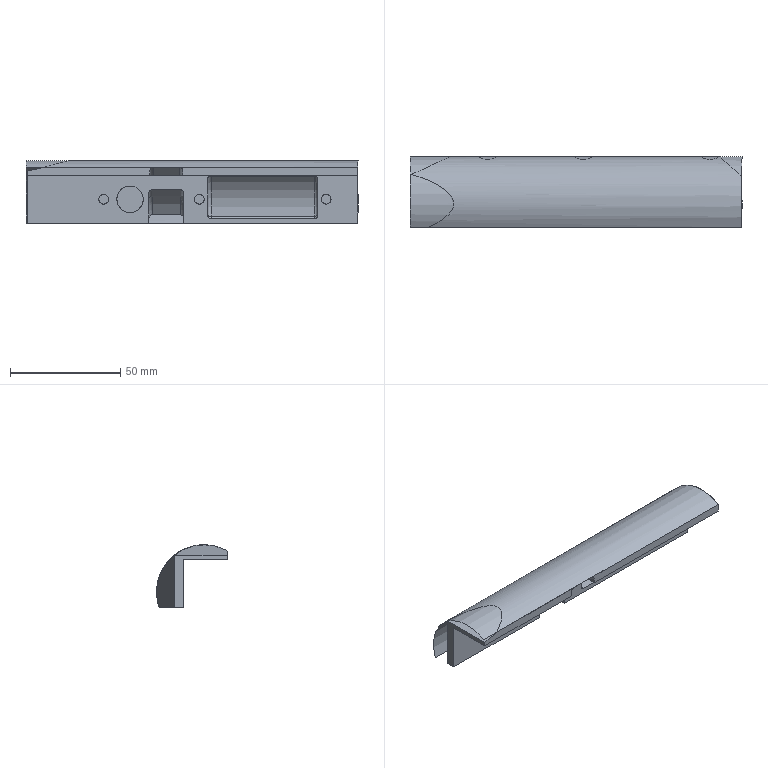CAM job | Mastercam | 3-axis milling, 5-axis milling, drilling
Tools:
tool_number,name,type,diameter_mm,corner_radius_mm,flutes,flute_length_mm,overall_length_mm,shoulder_length_mm,holder_diameter_mm,length_offset,diameter_offset,default_rpm,default_feed_mm_min,default_plunge_mm_min,coolant
1,3 Ball Mill / Bull Nose Mill,ball end mill,3,1.5,4,25,100,30,50,1,1,4000,480,600,COOL_OFF
4,4 Flat End Mill,end mill,4,0,4,25,75,25,50,4,4,6500,2000,600,COOL_OFF
5,4 Chamfer Mill,chamfer mill,4,0,4,25,75,30,50,5,5,6500,1000,600,COOL_OFF
9,10 Flat End Mill,end mill,10,0,4,25,75,25,50,9,9,6500,4000,600,COOL_OFF
10,10 Flat End Mill,end mill,10,0,4,25,75,25,50,10,10,6000,1000,600,COOL_OFF
14,3.3 Drill,drill,3.3,0,2,25,50,40,50,14,14,1818,218.16,600,COOL_OFF
15,4.4 Drill,drill,4.4,0,2,25,50,40,50,15,15,1000,120,600,COOL_OFF
17,6 Ball Mill / Bull Nose Mill,ball end mill,6,3,4,25,100,30,50,17,17,2000,240,600,COOL_OFF
18,10 Bull Nose Mill,bull end mill,10,1,4,25,100,25,50,18,18,1200,144,600,COOL_OFF
24,100 Flat End Mill,end mill,100,0,4,25,75,25,50,24,24,4000,1000,600,COOL_OFF
Operations:
seq,operation,operation_type,tool_number,tool_name,tool_diameter_mm,spindle_rpm,feed_mm_min,plunge_mm_min,retract_mm_min,cycle_time_s,wcs,posted,nc_file
1,Facing - [WCS: Plane] - [Tplane: Plane],Facing,24,100 Flat End Mill,100,4000,1000,600,1200,21.935,Plane,yes,.nc
2,2D High Speed (2D Dynamic Mill) - [WCS: Plane] - [Tplane: Plane],HighSpeed2D,9,10 Flat End Mill,10,6500,4000,600,1200,134.351,Plane,yes,.nc
3,3D High Speed (Area roughing) - [WCS: Plane] - [Tplane: Plane],HighSpeed3D,9,10 Flat End Mill,10,6500,4000,600,1200,359.186,Plane,yes,.nc
4,Contour (2D) - [WCS: Plane] - [Tplane: Plane],Contour,10,10 Flat End Mill,10,6000,1000,600,1200,39.407,Plane,yes,.nc
5,Contour (2D) - [WCS: Plane] - [Tplane: Plane],Contour,10,10 Flat End Mill,10,6000,300,600,1200,2.245,Plane,yes,.nc
6,Contour (2D) - [WCS: Plane] - [Tplane: Plane],Contour,10,10 Flat End Mill,10,6000,1000,600,1200,50.612,Plane,yes,.nc
7,Stock model - [WCS: Plane] - [Tplane: Plane] - 1,139,,,,0,0,0,0,0,Plane,yes,.nc
8,3D High Speed (Waterline rest passes) - [WCS: Plane] - [Tplane: Plane],HighSpeed3D,1,3 Ball Mill / Bull Nose Mill,3,6000,2000,600,1200,218.995,Plane,yes,.nc
9,3D High Speed (Waterline) - [WCS: Plane] - [Tplane: Plane],HighSpeed3D,1,3 Ball Mill / Bull Nose Mill,3,6000,3000,600,1200,33.056,Plane,yes,.nc
10,3D High Speed (Waterline) - [WCS: Plane] - [Tplane: Plane],HighSpeed3D,1,3 Ball Mill / Bull Nose Mill,3,6000,3000,600,1200,105.174,Plane,yes,.nc
11,Unified Guide - [WCS: Plane] - [Tplane: Plane],461,1,3 Ball Mill / Bull Nose Mill,3,6000,3000,600,1200,304.231,Plane,yes,.nc
12,Deburr 5-axis - [WCS: Plane] - [Tplane: Plane],459,1,3 Ball Mill / Bull Nose Mill,3,6000,1000,600,1200,35.278,Plane,yes,.nc
13,Contour (2D chamfer) - [WCS: Plane] - [Tplane: Plane],Contour,5,4 Chamfer Mill,4,6500,1000,600,1200,10.58,Plane,yes,.nc
14,Drill/Counterbore - [WCS: Plane] - [Tplane: Plane],Drill,5,4 Chamfer Mill,4,6000,200,600,1200,3.541,Plane,yes,.nc
15,Peck Drill - [WCS: Plane] - [Tplane: Plane],Drill,15,4.4 Drill,4.4,1000,120,600,1200,15.9,Plane,yes,.nc
16,Facing - [WCS: Plane-1] - [Tplane: Plane-1],Facing,24,100 Flat End Mill,100,4000,2000,600,1200,189.954,Plane-1,yes,.nc
17,Facing - [WCS: Plane-1] - [Tplane: Plane-1],Facing,10,10 Flat End Mill,10,6000,3000,600,1200,131.222,Plane-1,yes,.nc
18,Helix Bore - [WCS: Plane-1] - [Tplane: Plane-1],HelixBore,4,4 Flat End Mill,4,6500,2000,600,1200,28.927,Plane-1,yes,.nc
19,Contour (2D chamfer) - [WCS: Plane-1] - [Tplane: Plane-1],Contour,5,4 Chamfer Mill,4,6500,1000,600,1200,26.814,Plane-1,yes,.nc
20,Contour (2D chamfer) - [WCS: Plane-1] - [Tplane: Plane-1],Contour,5,4 Chamfer Mill,4,6500,1000,600,1200,3.01,Plane-1,yes,.nc
21,Stock model - [WCS: Plane-1] - [Tplane: Plane-1] - 2,139,,,,0,0,0,0,0,Plane-1,yes,.nc
22,3D High Speed (Dynamic OptiRough) - [WCS: Plane-4] - [Tplane: Plane-4],HighSpeed3D,9,10 Flat End Mill,10,6500,4000,600,1200,241.596,Plane-4,yes,.nc
23,Unified Flowline - [WCS: Plane-4] - [Tplane: Plane-4],461,17,6 Ball Mill / Bull Nose Mill,6,8000,4000,600,1200,788.405,Plane-4,yes,.nc
24,Unified Flowline - [WCS: Plane-4] - [Tplane: Plane-4],461,17,6 Ball Mill / Bull Nose Mill,6,8000,3000,600,1200,201.697,Plane-4,yes,.nc
25,Facing - [WCS: Plane-5] - [Tplane: Plane-5],Facing,24,100 Flat End Mill,100,4000,1000,600,1200,21.335,Plane-5,yes,.nc
26,Contour (Ramp) - [WCS: Plane-5] - [Tplane: Plane-5],Contour,9,10 Flat End Mill,10,7000,4000,600,1200,262.763,Plane-5,yes,.nc
27,Contour (2D) - [WCS: Plane-5] - [Tplane: Plane-5],Contour,10,10 Flat End Mill,10,7000,1000,600,1200,51.515,Plane-5,yes,.nc
28,Surface Finish Flowline - [WCS: Plane-5] - [Tplane: Plane-5],MultiSurfaceFinishFlowline,18,10 Bull Nose Mill,10,7000,4000,600,1200,164.405,Plane-5,yes,.nc
29,Drill/Counterbore - [WCS: Plane-5] - [Tplane: Plane-5],Drill,5,4 Chamfer Mill,4,6000,200,600,1200,2.966,Plane-5,yes,.nc
30,Peck Drill - [WCS: Plane-5] - [Tplane: Plane-5],Drill,14,3.3 Drill,3.3,1200,100,600,1200,21.888,Plane-5,yes,.nc
31,Contour (2D chamfer) - [WCS: Plane-5] - [Tplane: Plane-5],Contour,5,4 Chamfer Mill,4,6500,1000,600,1200,2.816,Plane-5,yes,.nc
32,Deburr 5-axis - [WCS: Plane-5] - [Tplane: Plane-5],459,1,3 Ball Mill / Bull Nose Mill,3,6000,1000,600,1200,14.398,Plane-5,yes,.nc
33,Facing - [WCS: Plane-6] - [Tplane: Plane-6],Facing,24,100 Flat End Mill,100,4000,3000,600,1200,86.373,Plane-6,yes,.nc
34,Surface Finish Flowline - [WCS: Plane-6] - [Tplane: Plane-6],MultiSurfaceFinishFlowline,18,10 Bull Nose Mill,10,7000,4000,600,1200,391.486,Plane-6,yes,.nc
35,Deburr 5-axis - [WCS: Plane-6] - [Tplane: Plane-6],459,1,3 Ball Mill / Bull Nose Mill,3,6000,1000,600,1200,7.718,Plane-6,yes,.nc